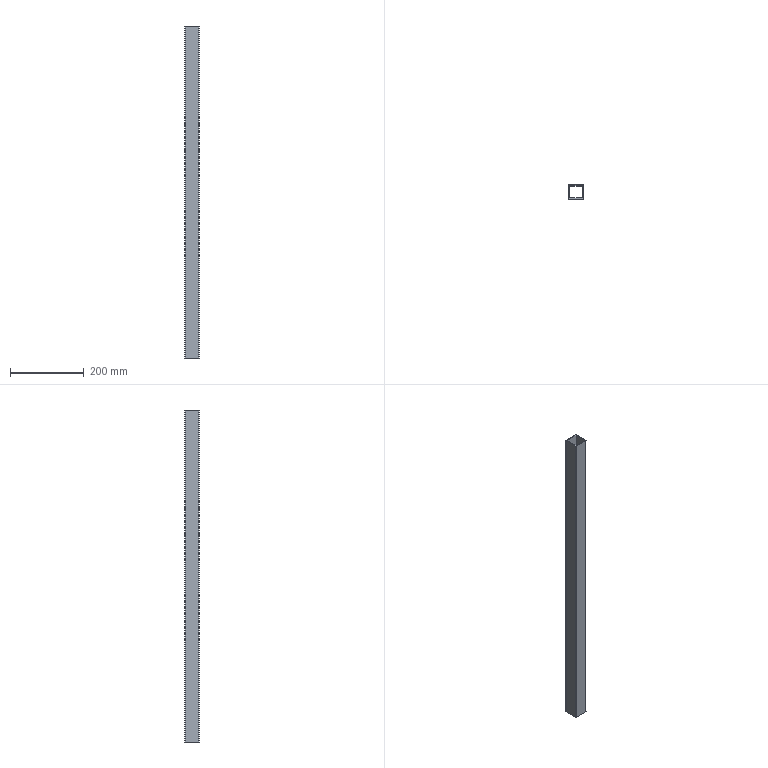Part | STEP file | X77-09103 | 1 solid | 14 faces | box 40 x 40 x 900 mm | volume 396510 mm3 | plane 10 | cylinder 4 | commonest cylinder face diameters 4 x4
STEP:
#1=CARTESIAN_POINT('',(0.,2.,900.));
#2=VERTEX_POINT('',#1);
#3=CARTESIAN_POINT('',(2.,0.,900.));
#4=VERTEX_POINT('',#3);
#5=CARTESIAN_POINT('',(2.,2.,900.));
#6=DIRECTION('',(0.,0.,1.));
#7=DIRECTION('',(1.,0.,0.));
#8=AXIS2_PLACEMENT_3D('',#5,#6,#7);
#9=CIRCLE('',#8,2.);
#10=EDGE_CURVE('',#2,#4,#9,.T.);
#11=ORIENTED_EDGE('',*,*,#10,.T.);
#12=CARTESIAN_POINT('',(38.,0.,900.));
#13=VERTEX_POINT('',#12);
#14=CARTESIAN_POINT('',(2.,0.,900.));
#15=DIRECTION('',(1.,0.,0.));
#16=VECTOR('',#15,1000.);
#17=LINE('',#14,#16);
#18=EDGE_CURVE('',#4,#13,#17,.T.);
#19=ORIENTED_EDGE('',*,*,#18,.T.);
#20=CARTESIAN_POINT('',(40.,2.,900.));
#21=VERTEX_POINT('',#20);
#22=CARTESIAN_POINT('',(38.,2.,900.));
#23=DIRECTION('',(0.,0.,1.));
#24=DIRECTION('',(1.,0.,0.));
#25=AXIS2_PLACEMENT_3D('',#22,#23,#24);
#26=CIRCLE('',#25,2.);
#27=EDGE_CURVE('',#13,#21,#26,.T.);
#28=ORIENTED_EDGE('',*,*,#27,.T.);
#29=CARTESIAN_POINT('',(40.,38.,900.));
#30=VERTEX_POINT('',#29);
#31=CARTESIAN_POINT('',(40.,2.,900.));
#32=DIRECTION('',(0.,1.,0.));
#33=VECTOR('',#32,1000.);
#34=LINE('',#31,#33);
#35=EDGE_CURVE('',#21,#30,#34,.T.);
#36=ORIENTED_EDGE('',*,*,#35,.T.);
#37=CARTESIAN_POINT('',(38.,40.,900.));
#38=VERTEX_POINT('',#37);
#39=CARTESIAN_POINT('',(38.,38.,900.));
#40=DIRECTION('',(0.,0.,1.));
#41=DIRECTION('',(1.,0.,0.));
#42=AXIS2_PLACEMENT_3D('',#39,#40,#41);
#43=CIRCLE('',#42,2.);
#44=EDGE_CURVE('',#30,#38,#43,.T.);
#45=ORIENTED_EDGE('',*,*,#44,.T.);
#46=CARTESIAN_POINT('',(2.,40.,900.));
#47=VERTEX_POINT('',#46);
#48=CARTESIAN_POINT('',(2.,40.,900.));
#49=DIRECTION('',(-1.,0.,0.));
#50=VECTOR('',#49,1000.);
#51=LINE('',#48,#50);
#52=EDGE_CURVE('',#38,#47,#51,.T.);
#53=ORIENTED_EDGE('',*,*,#52,.T.);
#54=CARTESIAN_POINT('',(0.,38.,900.));
#55=VERTEX_POINT('',#54);
#56=CARTESIAN_POINT('',(2.,38.,900.));
#57=DIRECTION('',(0.,0.,1.));
#58=DIRECTION('',(-1.,0.,0.));
#59=AXIS2_PLACEMENT_3D('',#56,#57,#58);
#60=CIRCLE('',#59,2.);
#61=EDGE_CURVE('',#47,#55,#60,.T.);
#62=ORIENTED_EDGE('',*,*,#61,.T.);
#63=CARTESIAN_POINT('',(0.,2.,900.));
#64=DIRECTION('',(0.,-1.,0.));
#65=VECTOR('',#64,1000.);
#66=LINE('',#63,#65);
#67=EDGE_CURVE('',#55,#2,#66,.T.);
#68=ORIENTED_EDGE('',*,*,#67,.T.);
#69=EDGE_LOOP('',(#11,#19,#28,#36,#45,#53,#62,#68));
#70=FACE_OUTER_BOUND('',#69,.T.);
#71=CARTESIAN_POINT('',(3.,3.,900.));
#72=VERTEX_POINT('',#71);
#73=CARTESIAN_POINT('',(37.,3.,900.));
#74=VERTEX_POINT('',#73);
#75=CARTESIAN_POINT('',(3.,3.,900.));
#76=DIRECTION('',(1.,0.,0.));
#77=VECTOR('',#76,1000.);
#78=LINE('',#75,#77);
#79=EDGE_CURVE('',#72,#74,#78,.T.);
#80=ORIENTED_EDGE('',*,*,#79,.F.);
#81=CARTESIAN_POINT('',(3.,37.,900.));
#82=VERTEX_POINT('',#81);
#83=CARTESIAN_POINT('',(3.,3.,900.));
#84=DIRECTION('',(0.,-1.,0.));
#85=VECTOR('',#84,1000.);
#86=LINE('',#83,#85);
#87=EDGE_CURVE('',#82,#72,#86,.T.);
#88=ORIENTED_EDGE('',*,*,#87,.F.);
#89=CARTESIAN_POINT('',(37.,37.,900.));
#90=VERTEX_POINT('',#89);
#91=CARTESIAN_POINT('',(3.,37.,900.));
#92=DIRECTION('',(-1.,0.,0.));
#93=VECTOR('',#92,1000.);
#94=LINE('',#91,#93);
#95=EDGE_CURVE('',#90,#82,#94,.T.);
#96=ORIENTED_EDGE('',*,*,#95,.F.);
#97=CARTESIAN_POINT('',(37.,3.,900.));
#98=DIRECTION('',(0.,1.,0.));
#99=VECTOR('',#98,1000.);
#100=LINE('',#97,#99);
#101=EDGE_CURVE('',#74,#90,#100,.T.);
#102=ORIENTED_EDGE('',*,*,#101,.F.);
#103=EDGE_LOOP('',(#80,#88,#96,#102));
#104=FACE_BOUND('',#103,.T.);
#105=CARTESIAN_POINT('',(2.,2.,900.));
#106=DIRECTION('',(0.,0.,1.));
#107=DIRECTION('',(1.,0.,0.));
#108=AXIS2_PLACEMENT_3D('',#105,#106,#107);
#109=PLANE('',#108);
#110=ADVANCED_FACE('',(#70,#104),#109,.T.);
#111=CARTESIAN_POINT('',(0.,2.,0.));
#112=VERTEX_POINT('',#111);
#113=CARTESIAN_POINT('',(2.,0.,0.));
#114=VERTEX_POINT('',#113);
#115=CARTESIAN_POINT('',(2.,2.,0.));
#116=DIRECTION('',(0.,0.,1.));
#117=DIRECTION('',(1.,0.,0.));
#118=AXIS2_PLACEMENT_3D('',#115,#116,#117);
#119=CIRCLE('',#118,2.);
#120=EDGE_CURVE('',#112,#114,#119,.T.);
#121=ORIENTED_EDGE('',*,*,#120,.F.);
#122=CARTESIAN_POINT('',(0.,38.,0.));
#123=VERTEX_POINT('',#122);
#124=CARTESIAN_POINT('',(0.,2.,0.));
#125=DIRECTION('',(0.,-1.,0.));
#126=VECTOR('',#125,1000.);
#127=LINE('',#124,#126);
#128=EDGE_CURVE('',#123,#112,#127,.T.);
#129=ORIENTED_EDGE('',*,*,#128,.F.);
#130=CARTESIAN_POINT('',(2.,40.,0.));
#131=VERTEX_POINT('',#130);
#132=CARTESIAN_POINT('',(2.,38.,0.));
#133=DIRECTION('',(0.,0.,1.));
#134=DIRECTION('',(-1.,0.,0.));
#135=AXIS2_PLACEMENT_3D('',#132,#133,#134);
#136=CIRCLE('',#135,2.);
#137=EDGE_CURVE('',#131,#123,#136,.T.);
#138=ORIENTED_EDGE('',*,*,#137,.F.);
#139=CARTESIAN_POINT('',(38.,40.,0.));
#140=VERTEX_POINT('',#139);
#141=CARTESIAN_POINT('',(2.,40.,0.));
#142=DIRECTION('',(-1.,0.,0.));
#143=VECTOR('',#142,1000.);
#144=LINE('',#141,#143);
#145=EDGE_CURVE('',#140,#131,#144,.T.);
#146=ORIENTED_EDGE('',*,*,#145,.F.);
#147=CARTESIAN_POINT('',(40.,38.,0.));
#148=VERTEX_POINT('',#147);
#149=CARTESIAN_POINT('',(38.,38.,0.));
#150=DIRECTION('',(0.,0.,1.));
#151=DIRECTION('',(1.,0.,0.));
#152=AXIS2_PLACEMENT_3D('',#149,#150,#151);
#153=CIRCLE('',#152,2.);
#154=EDGE_CURVE('',#148,#140,#153,.T.);
#155=ORIENTED_EDGE('',*,*,#154,.F.);
#156=CARTESIAN_POINT('',(40.,2.,0.));
#157=VERTEX_POINT('',#156);
#158=CARTESIAN_POINT('',(40.,2.,0.));
#159=DIRECTION('',(0.,1.,0.));
#160=VECTOR('',#159,1000.);
#161=LINE('',#158,#160);
#162=EDGE_CURVE('',#157,#148,#161,.T.);
#163=ORIENTED_EDGE('',*,*,#162,.F.);
#164=CARTESIAN_POINT('',(38.,0.,0.));
#165=VERTEX_POINT('',#164);
#166=CARTESIAN_POINT('',(38.,2.,0.));
#167=DIRECTION('',(0.,0.,1.));
#168=DIRECTION('',(1.,0.,0.));
#169=AXIS2_PLACEMENT_3D('',#166,#167,#168);
#170=CIRCLE('',#169,2.);
#171=EDGE_CURVE('',#165,#157,#170,.T.);
#172=ORIENTED_EDGE('',*,*,#171,.F.);
#173=CARTESIAN_POINT('',(2.,0.,0.));
#174=DIRECTION('',(1.,0.,0.));
#175=VECTOR('',#174,1000.);
#176=LINE('',#173,#175);
#177=EDGE_CURVE('',#114,#165,#176,.T.);
#178=ORIENTED_EDGE('',*,*,#177,.F.);
#179=EDGE_LOOP('',(#121,#129,#138,#146,#155,#163,#172,#178));
#180=FACE_OUTER_BOUND('',#179,.T.);
#181=CARTESIAN_POINT('',(3.,37.,0.));
#182=VERTEX_POINT('',#181);
#183=CARTESIAN_POINT('',(3.,3.,0.));
#184=VERTEX_POINT('',#183);
#185=CARTESIAN_POINT('',(3.,3.,0.));
#186=DIRECTION('',(0.,-1.,0.));
#187=VECTOR('',#186,1000.);
#188=LINE('',#185,#187);
#189=EDGE_CURVE('',#182,#184,#188,.T.);
#190=ORIENTED_EDGE('',*,*,#189,.T.);
#191=CARTESIAN_POINT('',(37.,3.,0.));
#192=VERTEX_POINT('',#191);
#193=CARTESIAN_POINT('',(3.,3.,0.));
#194=DIRECTION('',(1.,0.,0.));
#195=VECTOR('',#194,1000.);
#196=LINE('',#193,#195);
#197=EDGE_CURVE('',#184,#192,#196,.T.);
#198=ORIENTED_EDGE('',*,*,#197,.T.);
#199=CARTESIAN_POINT('',(37.,37.,0.));
#200=VERTEX_POINT('',#199);
#201=CARTESIAN_POINT('',(37.,3.,0.));
#202=DIRECTION('',(0.,1.,0.));
#203=VECTOR('',#202,1000.);
#204=LINE('',#201,#203);
#205=EDGE_CURVE('',#192,#200,#204,.T.);
#206=ORIENTED_EDGE('',*,*,#205,.T.);
#207=CARTESIAN_POINT('',(3.,37.,0.));
#208=DIRECTION('',(-1.,0.,0.));
#209=VECTOR('',#208,1000.);
#210=LINE('',#207,#209);
#211=EDGE_CURVE('',#200,#182,#210,.T.);
#212=ORIENTED_EDGE('',*,*,#211,.T.);
#213=EDGE_LOOP('',(#190,#198,#206,#212));
#214=FACE_BOUND('',#213,.T.);
#215=CARTESIAN_POINT('',(2.,2.,0.));
#216=DIRECTION('',(0.,0.,1.));
#217=DIRECTION('',(1.,0.,0.));
#218=AXIS2_PLACEMENT_3D('',#215,#216,#217);
#219=PLANE('',#218);
#220=ADVANCED_FACE('',(#180,#214),#219,.F.);
#221=ORIENTED_EDGE('',*,*,#120,.T.);
#222=CARTESIAN_POINT('',(2.,0.,900.));
#223=DIRECTION('',(0.,0.,-1.));
#224=VECTOR('',#223,1000.);
#225=LINE('',#222,#224);
#226=EDGE_CURVE('',#4,#114,#225,.T.);
#227=ORIENTED_EDGE('',*,*,#226,.F.);
#228=ORIENTED_EDGE('',*,*,#10,.F.);
#229=CARTESIAN_POINT('',(0.,2.,900.));
#230=DIRECTION('',(0.,0.,-1.));
#231=VECTOR('',#230,1000.);
#232=LINE('',#229,#231);
#233=EDGE_CURVE('',#2,#112,#232,.T.);
#234=ORIENTED_EDGE('',*,*,#233,.T.);
#235=EDGE_LOOP('',(#221,#227,#228,#234));
#236=FACE_OUTER_BOUND('',#235,.T.);
#237=CARTESIAN_POINT('',(2.,2.,900.));
#238=DIRECTION('',(0.,0.,-1.));
#239=DIRECTION('',(-1.,0.,0.));
#240=AXIS2_PLACEMENT_3D('',#237,#238,#239);
#241=CYLINDRICAL_SURFACE('',#240,2.);
#242=ADVANCED_FACE('',(#236),#241,.T.);
#243=ORIENTED_EDGE('',*,*,#177,.T.);
#244=CARTESIAN_POINT('',(38.,0.,900.));
#245=DIRECTION('',(0.,0.,-1.));
#246=VECTOR('',#245,1000.);
#247=LINE('',#244,#246);
#248=EDGE_CURVE('',#13,#165,#247,.T.);
#249=ORIENTED_EDGE('',*,*,#248,.F.);
#250=ORIENTED_EDGE('',*,*,#18,.F.);
#251=ORIENTED_EDGE('',*,*,#226,.T.);
#252=EDGE_LOOP('',(#243,#249,#250,#251));
#253=FACE_OUTER_BOUND('',#252,.T.);
#254=CARTESIAN_POINT('',(2.,0.,900.));
#255=DIRECTION('',(0.,1.,0.));
#256=DIRECTION('',(0.,0.,1.));
#257=AXIS2_PLACEMENT_3D('',#254,#255,#256);
#258=PLANE('',#257);
#259=ADVANCED_FACE('',(#253),#258,.F.);
#260=ORIENTED_EDGE('',*,*,#171,.T.);
#261=CARTESIAN_POINT('',(40.,2.,900.));
#262=DIRECTION('',(0.,0.,-1.));
#263=VECTOR('',#262,1000.);
#264=LINE('',#261,#263);
#265=EDGE_CURVE('',#21,#157,#264,.T.);
#266=ORIENTED_EDGE('',*,*,#265,.F.);
#267=ORIENTED_EDGE('',*,*,#27,.F.);
#268=ORIENTED_EDGE('',*,*,#248,.T.);
#269=EDGE_LOOP('',(#260,#266,#267,#268));
#270=FACE_OUTER_BOUND('',#269,.T.);
#271=CARTESIAN_POINT('',(38.,2.,900.));
#272=DIRECTION('',(0.,0.,-1.));
#273=DIRECTION('',(-1.,0.,0.));
#274=AXIS2_PLACEMENT_3D('',#271,#272,#273);
#275=CYLINDRICAL_SURFACE('',#274,2.);
#276=ADVANCED_FACE('',(#270),#275,.T.);
#277=ORIENTED_EDGE('',*,*,#162,.T.);
#278=CARTESIAN_POINT('',(40.,38.,900.));
#279=DIRECTION('',(0.,0.,-1.));
#280=VECTOR('',#279,1000.);
#281=LINE('',#278,#280);
#282=EDGE_CURVE('',#30,#148,#281,.T.);
#283=ORIENTED_EDGE('',*,*,#282,.F.);
#284=ORIENTED_EDGE('',*,*,#35,.F.);
#285=ORIENTED_EDGE('',*,*,#265,.T.);
#286=EDGE_LOOP('',(#277,#283,#284,#285));
#287=FACE_OUTER_BOUND('',#286,.T.);
#288=CARTESIAN_POINT('',(40.,2.,900.));
#289=DIRECTION('',(-1.,0.,0.));
#290=DIRECTION('',(0.,-1.,0.));
#291=AXIS2_PLACEMENT_3D('',#288,#289,#290);
#292=PLANE('',#291);
#293=ADVANCED_FACE('',(#287),#292,.F.);
#294=ORIENTED_EDGE('',*,*,#154,.T.);
#295=CARTESIAN_POINT('',(38.,40.,900.));
#296=DIRECTION('',(0.,0.,-1.));
#297=VECTOR('',#296,1000.);
#298=LINE('',#295,#297);
#299=EDGE_CURVE('',#38,#140,#298,.T.);
#300=ORIENTED_EDGE('',*,*,#299,.F.);
#301=ORIENTED_EDGE('',*,*,#44,.F.);
#302=ORIENTED_EDGE('',*,*,#282,.T.);
#303=EDGE_LOOP('',(#294,#300,#301,#302));
#304=FACE_OUTER_BOUND('',#303,.T.);
#305=CARTESIAN_POINT('',(38.,38.,900.));
#306=DIRECTION('',(0.,0.,-1.));
#307=DIRECTION('',(-1.,0.,0.));
#308=AXIS2_PLACEMENT_3D('',#305,#306,#307);
#309=CYLINDRICAL_SURFACE('',#308,2.);
#310=ADVANCED_FACE('',(#304),#309,.T.);
#311=ORIENTED_EDGE('',*,*,#145,.T.);
#312=CARTESIAN_POINT('',(2.,40.,900.));
#313=DIRECTION('',(0.,0.,-1.));
#314=VECTOR('',#313,1000.);
#315=LINE('',#312,#314);
#316=EDGE_CURVE('',#47,#131,#315,.T.);
#317=ORIENTED_EDGE('',*,*,#316,.F.);
#318=ORIENTED_EDGE('',*,*,#52,.F.);
#319=ORIENTED_EDGE('',*,*,#299,.T.);
#320=EDGE_LOOP('',(#311,#317,#318,#319));
#321=FACE_OUTER_BOUND('',#320,.T.);
#322=CARTESIAN_POINT('',(2.,40.,900.));
#323=DIRECTION('',(0.,-1.,0.));
#324=DIRECTION('',(0.,0.,-1.));
#325=AXIS2_PLACEMENT_3D('',#322,#323,#324);
#326=PLANE('',#325);
#327=ADVANCED_FACE('',(#321),#326,.F.);
#328=ORIENTED_EDGE('',*,*,#137,.T.);
#329=CARTESIAN_POINT('',(0.,38.,900.));
#330=DIRECTION('',(0.,0.,-1.));
#331=VECTOR('',#330,1000.);
#332=LINE('',#329,#331);
#333=EDGE_CURVE('',#55,#123,#332,.T.);
#334=ORIENTED_EDGE('',*,*,#333,.F.);
#335=ORIENTED_EDGE('',*,*,#61,.F.);
#336=ORIENTED_EDGE('',*,*,#316,.T.);
#337=EDGE_LOOP('',(#328,#334,#335,#336));
#338=FACE_OUTER_BOUND('',#337,.T.);
#339=CARTESIAN_POINT('',(2.,38.,900.));
#340=DIRECTION('',(0.,0.,-1.));
#341=DIRECTION('',(-1.,0.,0.));
#342=AXIS2_PLACEMENT_3D('',#339,#340,#341);
#343=CYLINDRICAL_SURFACE('',#342,2.);
#344=ADVANCED_FACE('',(#338),#343,.T.);
#345=ORIENTED_EDGE('',*,*,#128,.T.);
#346=ORIENTED_EDGE('',*,*,#233,.F.);
#347=ORIENTED_EDGE('',*,*,#67,.F.);
#348=ORIENTED_EDGE('',*,*,#333,.T.);
#349=EDGE_LOOP('',(#345,#346,#347,#348));
#350=FACE_OUTER_BOUND('',#349,.T.);
#351=CARTESIAN_POINT('',(0.,2.,900.));
#352=DIRECTION('',(1.,0.,0.));
#353=DIRECTION('',(0.,1.,0.));
#354=AXIS2_PLACEMENT_3D('',#351,#352,#353);
#355=PLANE('',#354);
#356=ADVANCED_FACE('',(#350),#355,.F.);
#357=ORIENTED_EDGE('',*,*,#189,.F.);
#358=CARTESIAN_POINT('',(3.,37.,900.));
#359=DIRECTION('',(0.,0.,-1.));
#360=VECTOR('',#359,1000.);
#361=LINE('',#358,#360);
#362=EDGE_CURVE('',#82,#182,#361,.T.);
#363=ORIENTED_EDGE('',*,*,#362,.F.);
#364=ORIENTED_EDGE('',*,*,#87,.T.);
#365=CARTESIAN_POINT('',(3.,3.,900.));
#366=DIRECTION('',(0.,0.,-1.));
#367=VECTOR('',#366,1000.);
#368=LINE('',#365,#367);
#369=EDGE_CURVE('',#72,#184,#368,.T.);
#370=ORIENTED_EDGE('',*,*,#369,.T.);
#371=EDGE_LOOP('',(#357,#363,#364,#370));
#372=FACE_OUTER_BOUND('',#371,.T.);
#373=CARTESIAN_POINT('',(3.,3.,900.));
#374=DIRECTION('',(1.,0.,0.));
#375=DIRECTION('',(0.,0.,-1.));
#376=AXIS2_PLACEMENT_3D('',#373,#374,#375);
#377=PLANE('',#376);
#378=ADVANCED_FACE('',(#372),#377,.T.);
#379=ORIENTED_EDGE('',*,*,#197,.F.);
#380=ORIENTED_EDGE('',*,*,#369,.F.);
#381=ORIENTED_EDGE('',*,*,#79,.T.);
#382=CARTESIAN_POINT('',(37.,3.,900.));
#383=DIRECTION('',(0.,0.,-1.));
#384=VECTOR('',#383,1000.);
#385=LINE('',#382,#384);
#386=EDGE_CURVE('',#74,#192,#385,.T.);
#387=ORIENTED_EDGE('',*,*,#386,.T.);
#388=EDGE_LOOP('',(#379,#380,#381,#387));
#389=FACE_OUTER_BOUND('',#388,.T.);
#390=CARTESIAN_POINT('',(3.,3.,900.));
#391=DIRECTION('',(0.,1.,0.));
#392=DIRECTION('',(0.,0.,1.));
#393=AXIS2_PLACEMENT_3D('',#390,#391,#392);
#394=PLANE('',#393);
#395=ADVANCED_FACE('',(#389),#394,.T.);
#396=ORIENTED_EDGE('',*,*,#205,.F.);
#397=ORIENTED_EDGE('',*,*,#386,.F.);
#398=ORIENTED_EDGE('',*,*,#101,.T.);
#399=CARTESIAN_POINT('',(37.,37.,900.));
#400=DIRECTION('',(0.,0.,-1.));
#401=VECTOR('',#400,1000.);
#402=LINE('',#399,#401);
#403=EDGE_CURVE('',#90,#200,#402,.T.);
#404=ORIENTED_EDGE('',*,*,#403,.T.);
#405=EDGE_LOOP('',(#396,#397,#398,#404));
#406=FACE_OUTER_BOUND('',#405,.T.);
#407=CARTESIAN_POINT('',(37.,3.,900.));
#408=DIRECTION('',(-1.,0.,0.));
#409=DIRECTION('',(0.,0.,1.));
#410=AXIS2_PLACEMENT_3D('',#407,#408,#409);
#411=PLANE('',#410);
#412=ADVANCED_FACE('',(#406),#411,.T.);
#413=ORIENTED_EDGE('',*,*,#211,.F.);
#414=ORIENTED_EDGE('',*,*,#403,.F.);
#415=ORIENTED_EDGE('',*,*,#95,.T.);
#416=ORIENTED_EDGE('',*,*,#362,.T.);
#417=EDGE_LOOP('',(#413,#414,#415,#416));
#418=FACE_OUTER_BOUND('',#417,.T.);
#419=CARTESIAN_POINT('',(3.,37.,900.));
#420=DIRECTION('',(0.,-1.,0.));
#421=DIRECTION('',(0.,0.,-1.));
#422=AXIS2_PLACEMENT_3D('',#419,#420,#421);
#423=PLANE('',#422);
#424=ADVANCED_FACE('',(#418),#423,.T.);
#425=CLOSED_SHELL('',(#110,#220,#242,#259,#276,#293,#310,#327,#344,#356,#378,#395,#412,#424));
#426=MANIFOLD_SOLID_BREP('',#425);
#427=CARTESIAN_POINT('',(0.,0.,0.));
#428=DIRECTION('',(0.,0.,1.));
#429=DIRECTION('',(1.,0.,0.));
#430=AXIS2_PLACEMENT_3D('',#427,#428,#429);
#431=(LENGTH_UNIT()NAMED_UNIT(*)SI_UNIT(.MILLI.,.METRE.));
#432=UNCERTAINTY_MEASURE_WITH_UNIT(LENGTH_MEASURE(0.00001),#431,'','');
#433=(NAMED_UNIT(*)PLANE_ANGLE_UNIT()SI_UNIT($,.RADIAN.));
#434=(NAMED_UNIT(*)SI_UNIT($,.STERADIAN.)SOLID_ANGLE_UNIT());
#435=(GEOMETRIC_REPRESENTATION_CONTEXT(3)GLOBAL_UNCERTAINTY_ASSIGNED_CONTEXT((#432))GLOBAL_UNIT_ASSIGNED_CONTEXT((#431,#433,#434))REPRESENTATION_CONTEXT('',''));
#436=ADVANCED_BREP_SHAPE_REPRESENTATION('',(#426,#430),#435);